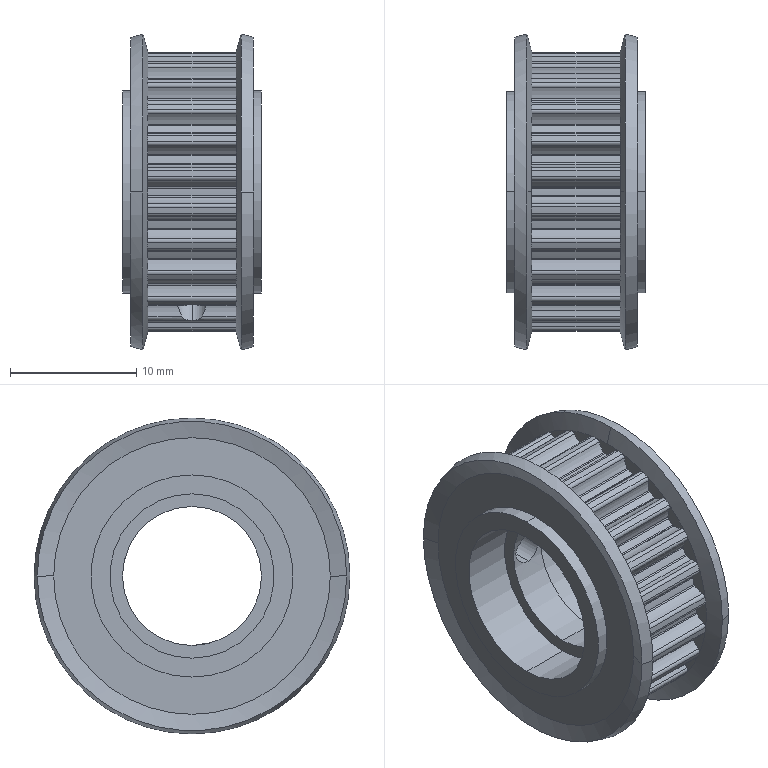Part | NX | features BREP 1 | 1 solid | 308 faces | box 11 x 25 x 25 mm | volume 2400 mm3 | cylinder 242 | plane 54 | cone 12 | commonest cylinder face diameters 0.56 x63 0.3 x58 3.95 x56 19.94 x27 22.16 x24 2.459 x4